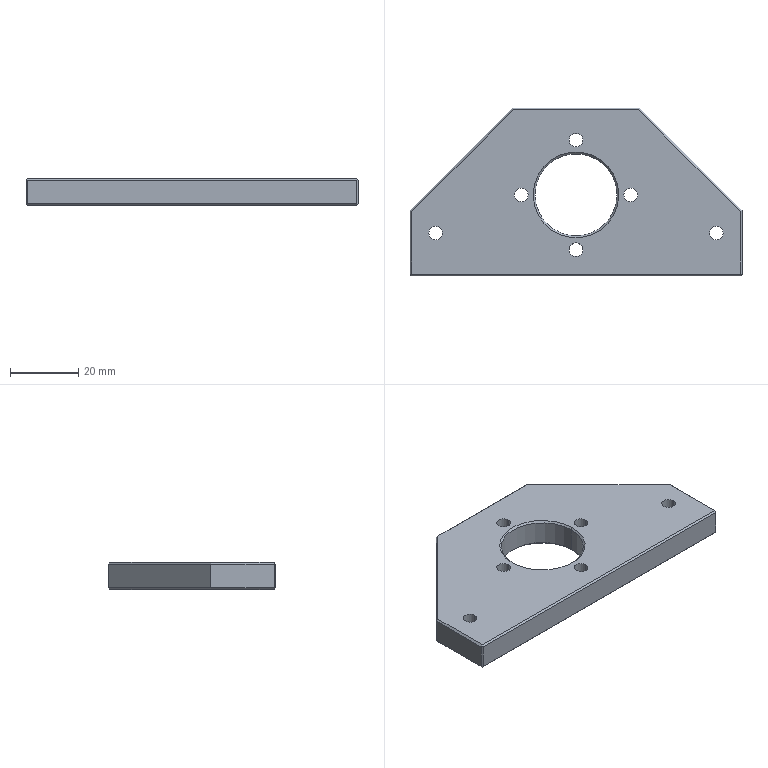Part | Creo | features DATUM PLANE 3, CURVE 2, CHAMFER 1, COORDINATE SYSTEM 1, CUT 1, PROTRUSION 1 | 1 solid | 46 faces | box 97 x 49 x 8 mm | volume 26205 mm3 | plane 24 | cylinder 18 | cone 4 | commonest cylinder face diameters 4 x12 7.464 x4 24 x2
STEP:
#1=CARTESIAN_POINT('',(0.,0.,0.));
#2=DIRECTION('',(0.,0.,1.));
#3=DIRECTION('',(1.,0.,0.));
#4=AXIS2_PLACEMENT_3D('',#1,#2,#3);
#5=CARTESIAN_POINT('',(48.,0.5,0.));
#6=VERTEX_POINT('',#5);
#7=CARTESIAN_POINT('',(-48.,0.5,0.));
#8=VERTEX_POINT('',#7);
#9=CARTESIAN_POINT('',(48.,0.5,0.));
#10=DIRECTION('',(-1.,0.,0.));
#11=VECTOR('',#10,96.);
#12=LINE('',#9,#11);
#13=EDGE_CURVE('',#6,#8,#12,.T.);
#14=ORIENTED_EDGE('',*,*,#13,.F.);
#15=CARTESIAN_POINT('',(48.,18.793,0.));
#16=VERTEX_POINT('',#15);
#17=CARTESIAN_POINT('',(48.,18.793,0.));
#18=DIRECTION('',(0.,-1.,0.));
#19=VECTOR('',#18,18.293);
#20=LINE('',#17,#19);
#21=EDGE_CURVE('',#16,#6,#20,.T.);
#22=ORIENTED_EDGE('',*,*,#21,.F.);
#23=CARTESIAN_POINT('',(18.293,48.5,0.));
#24=VERTEX_POINT('',#23);
#25=CARTESIAN_POINT('',(18.293,48.5,0.));
#26=DIRECTION('',(0.7071,-0.7071,0.));
#27=VECTOR('',#26,42.012);
#28=LINE('',#25,#27);
#29=EDGE_CURVE('',#24,#16,#28,.T.);
#30=ORIENTED_EDGE('',*,*,#29,.F.);
#31=CARTESIAN_POINT('',(-18.293,48.5,0.));
#32=VERTEX_POINT('',#31);
#33=CARTESIAN_POINT('',(-18.293,48.5,0.));
#34=DIRECTION('',(1.,0.,0.));
#35=VECTOR('',#34,36.586);
#36=LINE('',#33,#35);
#37=EDGE_CURVE('',#32,#24,#36,.T.);
#38=ORIENTED_EDGE('',*,*,#37,.F.);
#39=CARTESIAN_POINT('',(-48.,18.793,0.));
#40=VERTEX_POINT('',#39);
#41=CARTESIAN_POINT('',(-48.,18.793,0.));
#42=DIRECTION('',(0.7071,0.7071,0.));
#43=VECTOR('',#42,42.012);
#44=LINE('',#41,#43);
#45=EDGE_CURVE('',#40,#32,#44,.T.);
#46=ORIENTED_EDGE('',*,*,#45,.F.);
#47=CARTESIAN_POINT('',(-48.,0.5,0.));
#48=DIRECTION('',(0.,1.,0.));
#49=VECTOR('',#48,18.293);
#50=LINE('',#47,#49);
#51=EDGE_CURVE('',#8,#40,#50,.T.);
#52=ORIENTED_EDGE('',*,*,#51,.F.);
#53=EDGE_LOOP('',(#14,#22,#30,#38,#46,#52));
#54=FACE_OUTER_BOUND('',#53,.F.);
#55=CARTESIAN_POINT('',(2.,39.66,0.));
#56=VERTEX_POINT('',#55);
#57=CARTESIAN_POINT('',(-2.,39.66,0.));
#58=VERTEX_POINT('',#57);
#59=CARTESIAN_POINT('',(0.,39.66,0.));
#60=DIRECTION('',(0.,0.,-1.));
#61=DIRECTION('',(1.,0.,0.));
#62=AXIS2_PLACEMENT_3D('',#59,#60,#61);
#63=CIRCLE('',#62,2.);
#64=EDGE_CURVE('',#56,#58,#63,.T.);
#65=ORIENTED_EDGE('',*,*,#64,.T.);
#66=CARTESIAN_POINT('',(0.,39.66,0.));
#67=DIRECTION('',(0.,0.,-1.));
#68=DIRECTION('',(-1.,0.,0.));
#69=AXIS2_PLACEMENT_3D('',#66,#67,#68);
#70=CIRCLE('',#69,2.);
#71=EDGE_CURVE('',#58,#56,#70,.T.);
#72=ORIENTED_EDGE('',*,*,#71,.T.);
#73=EDGE_LOOP('',(#65,#72));
#74=FACE_BOUND('',#73,.F.);
#75=CARTESIAN_POINT('',(-14.,23.66,0.));
#76=VERTEX_POINT('',#75);
#77=CARTESIAN_POINT('',(-18.,23.66,0.));
#78=VERTEX_POINT('',#77);
#79=CARTESIAN_POINT('',(-16.,23.66,0.));
#80=DIRECTION('',(0.,0.,-1.));
#81=DIRECTION('',(1.,0.,0.));
#82=AXIS2_PLACEMENT_3D('',#79,#80,#81);
#83=CIRCLE('',#82,2.);
#84=EDGE_CURVE('',#76,#78,#83,.T.);
#85=ORIENTED_EDGE('',*,*,#84,.T.);
#86=CARTESIAN_POINT('',(-16.,23.66,0.));
#87=DIRECTION('',(0.,0.,-1.));
#88=DIRECTION('',(-1.,0.,0.));
#89=AXIS2_PLACEMENT_3D('',#86,#87,#88);
#90=CIRCLE('',#89,2.);
#91=EDGE_CURVE('',#78,#76,#90,.T.);
#92=ORIENTED_EDGE('',*,*,#91,.T.);
#93=EDGE_LOOP('',(#85,#92));
#94=FACE_BOUND('',#93,.F.);
#95=CARTESIAN_POINT('',(2.,7.66,0.));
#96=VERTEX_POINT('',#95);
#97=CARTESIAN_POINT('',(-2.,7.66,0.));
#98=VERTEX_POINT('',#97);
#99=CARTESIAN_POINT('',(0.,7.66,0.));
#100=DIRECTION('',(0.,0.,-1.));
#101=DIRECTION('',(1.,0.,0.));
#102=AXIS2_PLACEMENT_3D('',#99,#100,#101);
#103=CIRCLE('',#102,2.);
#104=EDGE_CURVE('',#96,#98,#103,.T.);
#105=ORIENTED_EDGE('',*,*,#104,.T.);
#106=CARTESIAN_POINT('',(0.,7.66,0.));
#107=DIRECTION('',(0.,0.,-1.));
#108=DIRECTION('',(-1.,0.,0.));
#109=AXIS2_PLACEMENT_3D('',#106,#107,#108);
#110=CIRCLE('',#109,2.);
#111=EDGE_CURVE('',#98,#96,#110,.T.);
#112=ORIENTED_EDGE('',*,*,#111,.T.);
#113=EDGE_LOOP('',(#105,#112));
#114=FACE_BOUND('',#113,.F.);
#115=CARTESIAN_POINT('',(-44.732,12.5,0.));
#116=VERTEX_POINT('',#115);
#117=CARTESIAN_POINT('',(-37.268,12.5,0.));
#118=VERTEX_POINT('',#117);
#119=CARTESIAN_POINT('',(-41.,12.5,0.));
#120=DIRECTION('',(0.,0.,-1.));
#121=DIRECTION('',(-1.,0.,0.));
#122=AXIS2_PLACEMENT_3D('',#119,#120,#121);
#123=CIRCLE('',#122,3.732);
#124=EDGE_CURVE('',#116,#118,#123,.T.);
#125=ORIENTED_EDGE('',*,*,#124,.T.);
#126=CARTESIAN_POINT('',(-41.,12.5,0.));
#127=DIRECTION('',(0.,0.,-1.));
#128=DIRECTION('',(1.,0.,0.));
#129=AXIS2_PLACEMENT_3D('',#126,#127,#128);
#130=CIRCLE('',#129,3.732);
#131=EDGE_CURVE('',#118,#116,#130,.T.);
#132=ORIENTED_EDGE('',*,*,#131,.T.);
#133=EDGE_LOOP('',(#125,#132));
#134=FACE_BOUND('',#133,.F.);
#135=CARTESIAN_POINT('',(37.268,12.5,0.));
#136=VERTEX_POINT('',#135);
#137=CARTESIAN_POINT('',(44.732,12.5,0.));
#138=VERTEX_POINT('',#137);
#139=CARTESIAN_POINT('',(41.,12.5,0.));
#140=DIRECTION('',(0.,0.,-1.));
#141=DIRECTION('',(-1.,0.,0.));
#142=AXIS2_PLACEMENT_3D('',#139,#140,#141);
#143=CIRCLE('',#142,3.732);
#144=EDGE_CURVE('',#136,#138,#143,.T.);
#145=ORIENTED_EDGE('',*,*,#144,.T.);
#146=CARTESIAN_POINT('',(41.,12.5,0.));
#147=DIRECTION('',(0.,0.,-1.));
#148=DIRECTION('',(1.,0.,0.));
#149=AXIS2_PLACEMENT_3D('',#146,#147,#148);
#150=CIRCLE('',#149,3.732);
#151=EDGE_CURVE('',#138,#136,#150,.T.);
#152=ORIENTED_EDGE('',*,*,#151,.T.);
#153=EDGE_LOOP('',(#145,#152));
#154=FACE_BOUND('',#153,.F.);
#155=CARTESIAN_POINT('',(18.,23.66,0.));
#156=VERTEX_POINT('',#155);
#157=CARTESIAN_POINT('',(14.,23.66,0.));
#158=VERTEX_POINT('',#157);
#159=CARTESIAN_POINT('',(16.,23.66,0.));
#160=DIRECTION('',(0.,0.,-1.));
#161=DIRECTION('',(1.,0.,0.));
#162=AXIS2_PLACEMENT_3D('',#159,#160,#161);
#163=CIRCLE('',#162,2.);
#164=EDGE_CURVE('',#156,#158,#163,.T.);
#165=ORIENTED_EDGE('',*,*,#164,.T.);
#166=CARTESIAN_POINT('',(16.,23.66,0.));
#167=DIRECTION('',(0.,0.,-1.));
#168=DIRECTION('',(-1.,0.,0.));
#169=AXIS2_PLACEMENT_3D('',#166,#167,#168);
#170=CIRCLE('',#169,2.);
#171=EDGE_CURVE('',#158,#156,#170,.T.);
#172=ORIENTED_EDGE('',*,*,#171,.T.);
#173=EDGE_LOOP('',(#165,#172));
#174=FACE_BOUND('',#173,.F.);
#175=CARTESIAN_POINT('',(12.5,23.66,0.));
#176=VERTEX_POINT('',#175);
#177=CARTESIAN_POINT('',(-12.5,23.66,0.));
#178=VERTEX_POINT('',#177);
#179=CARTESIAN_POINT('',(0.,23.66,0.));
#180=DIRECTION('',(0.,0.,1.));
#181=DIRECTION('',(1.,0.,0.));
#182=AXIS2_PLACEMENT_3D('',#179,#180,#181);
#183=CIRCLE('',#182,12.5);
#184=EDGE_CURVE('',#176,#178,#183,.T.);
#185=ORIENTED_EDGE('',*,*,#184,.F.);
#186=CARTESIAN_POINT('',(0.,23.66,0.));
#187=DIRECTION('',(0.,0.,1.));
#188=DIRECTION('',(-1.,0.,0.));
#189=AXIS2_PLACEMENT_3D('',#186,#187,#188);
#190=CIRCLE('',#189,12.5);
#191=EDGE_CURVE('',#178,#176,#190,.T.);
#192=ORIENTED_EDGE('',*,*,#191,.F.);
#193=EDGE_LOOP('',(#185,#192));
#194=FACE_BOUND('',#193,.F.);
#195=CARTESIAN_POINT('',(0.,0.,0.));
#196=DIRECTION('',(0.,0.,1.));
#197=DIRECTION('',(1.,0.,0.));
#198=AXIS2_PLACEMENT_3D('',#195,#196,#197);
#199=PLANE('',#198);
#200=ADVANCED_FACE('',(#54,#74,#94,#114,#134,#154,#174,#194),#199,.F.);
#201=ORIENTED_EDGE('',*,*,#164,.F.);
#202=CARTESIAN_POINT('',(18.,23.66,8.));
#203=VERTEX_POINT('',#202);
#204=CARTESIAN_POINT('',(18.,23.66,0.));
#205=DIRECTION('',(0.,0.,1.));
#206=VECTOR('',#205,8.);
#207=LINE('',#204,#206);
#208=EDGE_CURVE('',#156,#203,#207,.T.);
#209=ORIENTED_EDGE('',*,*,#208,.T.);
#210=CARTESIAN_POINT('',(14.,23.66,8.));
#211=VERTEX_POINT('',#210);
#212=CARTESIAN_POINT('',(16.,23.66,8.));
#213=DIRECTION('',(0.,0.,-1.));
#214=DIRECTION('',(1.,0.,0.));
#215=AXIS2_PLACEMENT_3D('',#212,#213,#214);
#216=CIRCLE('',#215,2.);
#217=EDGE_CURVE('',#203,#211,#216,.T.);
#218=ORIENTED_EDGE('',*,*,#217,.T.);
#219=CARTESIAN_POINT('',(14.,23.66,0.));
#220=DIRECTION('',(0.,0.,1.));
#221=VECTOR('',#220,8.);
#222=LINE('',#219,#221);
#223=EDGE_CURVE('',#158,#211,#222,.T.);
#224=ORIENTED_EDGE('',*,*,#223,.F.);
#225=EDGE_LOOP('',(#201,#209,#218,#224));
#226=FACE_OUTER_BOUND('',#225,.F.);
#227=CARTESIAN_POINT('',(16.,23.66,0.));
#228=DIRECTION('',(0.,0.,1.));
#229=DIRECTION('',(1.,0.,0.));
#230=AXIS2_PLACEMENT_3D('',#227,#228,#229);
#231=CYLINDRICAL_SURFACE('',#230,2.);
#232=ADVANCED_FACE('',(#226),#231,.F.);
#233=ORIENTED_EDGE('',*,*,#171,.F.);
#234=ORIENTED_EDGE('',*,*,#223,.T.);
#235=CARTESIAN_POINT('',(16.,23.66,8.));
#236=DIRECTION('',(0.,0.,-1.));
#237=DIRECTION('',(-1.,0.,0.));
#238=AXIS2_PLACEMENT_3D('',#235,#236,#237);
#239=CIRCLE('',#238,2.);
#240=EDGE_CURVE('',#211,#203,#239,.T.);
#241=ORIENTED_EDGE('',*,*,#240,.T.);
#242=ORIENTED_EDGE('',*,*,#208,.F.);
#243=EDGE_LOOP('',(#233,#234,#241,#242));
#244=FACE_OUTER_BOUND('',#243,.F.);
#245=CARTESIAN_POINT('',(16.,23.66,0.));
#246=DIRECTION('',(0.,0.,1.));
#247=DIRECTION('',(1.,0.,0.));
#248=AXIS2_PLACEMENT_3D('',#245,#246,#247);
#249=CYLINDRICAL_SURFACE('',#248,2.);
#250=ADVANCED_FACE('',(#244),#249,.F.);
#251=CARTESIAN_POINT('',(-48.,0.5,8.));
#252=VERTEX_POINT('',#251);
#253=CARTESIAN_POINT('',(48.,0.5,8.));
#254=VERTEX_POINT('',#253);
#255=CARTESIAN_POINT('',(-48.,0.5,8.));
#256=DIRECTION('',(1.,0.,0.));
#257=VECTOR('',#256,96.);
#258=LINE('',#255,#257);
#259=EDGE_CURVE('',#252,#254,#258,.T.);
#260=ORIENTED_EDGE('',*,*,#259,.F.);
#261=CARTESIAN_POINT('',(-48.,18.793,8.));
#262=VERTEX_POINT('',#261);
#263=CARTESIAN_POINT('',(-48.,18.793,8.));
#264=DIRECTION('',(0.,-1.,0.));
#265=VECTOR('',#264,18.293);
#266=LINE('',#263,#265);
#267=EDGE_CURVE('',#262,#252,#266,.T.);
#268=ORIENTED_EDGE('',*,*,#267,.F.);
#269=CARTESIAN_POINT('',(-18.293,48.5,8.));
#270=VERTEX_POINT('',#269);
#271=CARTESIAN_POINT('',(-18.293,48.5,8.));
#272=DIRECTION('',(-0.7071,-0.7071,0.));
#273=VECTOR('',#272,42.012);
#274=LINE('',#271,#273);
#275=EDGE_CURVE('',#270,#262,#274,.T.);
#276=ORIENTED_EDGE('',*,*,#275,.F.);
#277=CARTESIAN_POINT('',(18.293,48.5,8.));
#278=VERTEX_POINT('',#277);
#279=CARTESIAN_POINT('',(18.293,48.5,8.));
#280=DIRECTION('',(-1.,0.,0.));
#281=VECTOR('',#280,36.586);
#282=LINE('',#279,#281);
#283=EDGE_CURVE('',#278,#270,#282,.T.);
#284=ORIENTED_EDGE('',*,*,#283,.F.);
#285=CARTESIAN_POINT('',(48.,18.793,8.));
#286=VERTEX_POINT('',#285);
#287=CARTESIAN_POINT('',(48.,18.793,8.));
#288=DIRECTION('',(-0.7071,0.7071,0.));
#289=VECTOR('',#288,42.012);
#290=LINE('',#287,#289);
#291=EDGE_CURVE('',#286,#278,#290,.T.);
#292=ORIENTED_EDGE('',*,*,#291,.F.);
#293=CARTESIAN_POINT('',(48.,0.5,8.));
#294=DIRECTION('',(0.,1.,0.));
#295=VECTOR('',#294,18.293);
#296=LINE('',#293,#295);
#297=EDGE_CURVE('',#254,#286,#296,.T.);
#298=ORIENTED_EDGE('',*,*,#297,.F.);
#299=EDGE_LOOP('',(#260,#268,#276,#284,#292,#298));
#300=FACE_OUTER_BOUND('',#299,.F.);
#301=CARTESIAN_POINT('',(43.,12.5,8.));
#302=VERTEX_POINT('',#301);
#303=CARTESIAN_POINT('',(39.,12.5,8.));
#304=VERTEX_POINT('',#303);
#305=CARTESIAN_POINT('',(41.,12.5,8.));
#306=DIRECTION('',(0.,0.,-1.));
#307=DIRECTION('',(1.,0.,0.));
#308=AXIS2_PLACEMENT_3D('',#305,#306,#307);
#309=CIRCLE('',#308,2.);
#310=EDGE_CURVE('',#302,#304,#309,.T.);
#311=ORIENTED_EDGE('',*,*,#310,.F.);
#312=CARTESIAN_POINT('',(41.,12.5,8.));
#313=DIRECTION('',(0.,0.,-1.));
#314=DIRECTION('',(-1.,0.,0.));
#315=AXIS2_PLACEMENT_3D('',#312,#313,#314);
#316=CIRCLE('',#315,2.);
#317=EDGE_CURVE('',#304,#302,#316,.T.);
#318=ORIENTED_EDGE('',*,*,#317,.F.);
#319=EDGE_LOOP('',(#311,#318));
#320=FACE_BOUND('',#319,.F.);
#321=ORIENTED_EDGE('',*,*,#217,.F.);
#322=ORIENTED_EDGE('',*,*,#240,.F.);
#323=EDGE_LOOP('',(#321,#322));
#324=FACE_BOUND('',#323,.F.);
#325=CARTESIAN_POINT('',(2.,39.66,8.));
#326=VERTEX_POINT('',#325);
#327=CARTESIAN_POINT('',(-2.,39.66,8.));
#328=VERTEX_POINT('',#327);
#329=CARTESIAN_POINT('',(0.,39.66,8.));
#330=DIRECTION('',(0.,0.,-1.));
#331=DIRECTION('',(1.,0.,0.));
#332=AXIS2_PLACEMENT_3D('',#329,#330,#331);
#333=CIRCLE('',#332,2.);
#334=EDGE_CURVE('',#326,#328,#333,.T.);
#335=ORIENTED_EDGE('',*,*,#334,.F.);
#336=CARTESIAN_POINT('',(0.,39.66,8.));
#337=DIRECTION('',(0.,0.,-1.));
#338=DIRECTION('',(-1.,0.,0.));
#339=AXIS2_PLACEMENT_3D('',#336,#337,#338);
#340=CIRCLE('',#339,2.);
#341=EDGE_CURVE('',#328,#326,#340,.T.);
#342=ORIENTED_EDGE('',*,*,#341,.F.);
#343=EDGE_LOOP('',(#335,#342));
#344=FACE_BOUND('',#343,.F.);
#345=CARTESIAN_POINT('',(-14.,23.66,8.));
#346=VERTEX_POINT('',#345);
#347=CARTESIAN_POINT('',(-18.,23.66,8.));
#348=VERTEX_POINT('',#347);
#349=CARTESIAN_POINT('',(-16.,23.66,8.));
#350=DIRECTION('',(0.,0.,-1.));
#351=DIRECTION('',(1.,0.,0.));
#352=AXIS2_PLACEMENT_3D('',#349,#350,#351);
#353=CIRCLE('',#352,2.);
#354=EDGE_CURVE('',#346,#348,#353,.T.);
#355=ORIENTED_EDGE('',*,*,#354,.F.);
#356=CARTESIAN_POINT('',(-16.,23.66,8.));
#357=DIRECTION('',(0.,0.,-1.));
#358=DIRECTION('',(-1.,0.,0.));
#359=AXIS2_PLACEMENT_3D('',#356,#357,#358);
#360=CIRCLE('',#359,2.);
#361=EDGE_CURVE('',#348,#346,#360,.T.);
#362=ORIENTED_EDGE('',*,*,#361,.F.);
#363=EDGE_LOOP('',(#355,#362));
#364=FACE_BOUND('',#363,.F.);
#365=CARTESIAN_POINT('',(2.,7.66,8.));
#366=VERTEX_POINT('',#365);
#367=CARTESIAN_POINT('',(-2.,7.66,8.));
#368=VERTEX_POINT('',#367);
#369=CARTESIAN_POINT('',(0.,7.66,8.));
#370=DIRECTION('',(0.,0.,-1.));
#371=DIRECTION('',(1.,0.,0.));
#372=AXIS2_PLACEMENT_3D('',#369,#370,#371);
#373=CIRCLE('',#372,2.);
#374=EDGE_CURVE('',#366,#368,#373,.T.);
#375=ORIENTED_EDGE('',*,*,#374,.F.);
#376=CARTESIAN_POINT('',(0.,7.66,8.));
#377=DIRECTION('',(0.,0.,-1.));
#378=DIRECTION('',(-1.,0.,0.));
#379=AXIS2_PLACEMENT_3D('',#376,#377,#378);
#380=CIRCLE('',#379,2.);
#381=EDGE_CURVE('',#368,#366,#380,.T.);
#382=ORIENTED_EDGE('',*,*,#381,.F.);
#383=EDGE_LOOP('',(#375,#382));
#384=FACE_BOUND('',#383,.F.);
#385=CARTESIAN_POINT('',(-39.,12.5,8.));
#386=VERTEX_POINT('',#385);
#387=CARTESIAN_POINT('',(-43.,12.5,8.));
#388=VERTEX_POINT('',#387);
#389=CARTESIAN_POINT('',(-41.,12.5,8.));
#390=DIRECTION('',(0.,0.,-1.));
#391=DIRECTION('',(1.,0.,0.));
#392=AXIS2_PLACEMENT_3D('',#389,#390,#391);
#393=CIRCLE('',#392,2.);
#394=EDGE_CURVE('',#386,#388,#393,.T.);
#395=ORIENTED_EDGE('',*,*,#394,.F.);
#396=CARTESIAN_POINT('',(-41.,12.5,8.));
#397=DIRECTION('',(0.,0.,-1.));
#398=DIRECTION('',(-1.,0.,0.));
#399=AXIS2_PLACEMENT_3D('',#396,#397,#398);
#400=CIRCLE('',#399,2.);
#401=EDGE_CURVE('',#388,#386,#400,.T.);
#402=ORIENTED_EDGE('',*,*,#401,.F.);
#403=EDGE_LOOP('',(#395,#402));
#404=FACE_BOUND('',#403,.F.);
#405=CARTESIAN_POINT('',(-12.5,23.66,8.));
#406=VERTEX_POINT('',#405);
#407=CARTESIAN_POINT('',(12.5,23.66,8.));
#408=VERTEX_POINT('',#407);
#409=CARTESIAN_POINT('',(0.,23.66,8.));
#410=DIRECTION('',(0.,0.,-1.));
#411=DIRECTION('',(-1.,0.,0.));
#412=AXIS2_PLACEMENT_3D('',#409,#410,#411);
#413=CIRCLE('',#412,12.5);
#414=EDGE_CURVE('',#406,#408,#413,.T.);
#415=ORIENTED_EDGE('',*,*,#414,.F.);
#416=CARTESIAN_POINT('',(0.,23.66,8.));
#417=DIRECTION('',(0.,0.,-1.));
#418=DIRECTION('',(1.,0.,0.));
#419=AXIS2_PLACEMENT_3D('',#416,#417,#418);
#420=CIRCLE('',#419,12.5);
#421=EDGE_CURVE('',#408,#406,#420,.T.);
#422=ORIENTED_EDGE('',*,*,#421,.F.);
#423=EDGE_LOOP('',(#415,#422));
#424=FACE_BOUND('',#423,.F.);
#425=CARTESIAN_POINT('',(0.,0.,8.));
#426=DIRECTION('',(0.,0.,1.));
#427=DIRECTION('',(1.,0.,0.));
#428=AXIS2_PLACEMENT_3D('',#425,#426,#427);
#429=PLANE('',#428);
#430=ADVANCED_FACE('',(#300,#320,#324,#344,#364,#384,#404,#424),#429,.T.);
#431=CARTESIAN_POINT('',(-43.,12.5,5.));
#432=VERTEX_POINT('',#431);
#433=CARTESIAN_POINT('',(-39.,12.5,5.));
#434=VERTEX_POINT('',#433);
#435=CARTESIAN_POINT('',(-41.,12.5,5.));
#436=DIRECTION('',(0.,0.,1.));
#437=DIRECTION('',(-1.,0.,0.));
#438=AXIS2_PLACEMENT_3D('',#435,#436,#437);
#439=CIRCLE('',#438,2.);
#440=EDGE_CURVE('',#432,#434,#439,.T.);
#441=ORIENTED_EDGE('',*,*,#440,.T.);
#442=CARTESIAN_POINT('',(-39.,12.5,5.));
#443=DIRECTION('',(0.,0.,1.));
#444=VECTOR('',#443,3.);
#445=LINE('',#442,#444);
#446=EDGE_CURVE('',#434,#386,#445,.T.);
#447=ORIENTED_EDGE('',*,*,#446,.T.);
#448=ORIENTED_EDGE('',*,*,#394,.T.);
#449=CARTESIAN_POINT('',(-43.,12.5,5.));
#450=DIRECTION('',(0.,0.,1.));
#451=VECTOR('',#450,3.);
#452=LINE('',#449,#451);
#453=EDGE_CURVE('',#432,#388,#452,.T.);
#454=ORIENTED_EDGE('',*,*,#453,.F.);
#455=EDGE_LOOP('',(#441,#447,#448,#454));
#456=FACE_OUTER_BOUND('',#455,.F.);
#457=CARTESIAN_POINT('',(-41.,12.5,0.));
#458=DIRECTION('',(0.,0.,1.));
#459=DIRECTION('',(1.,0.,0.));
#460=AXIS2_PLACEMENT_3D('',#457,#458,#459);
#461=CYLINDRICAL_SURFACE('',#460,2.);
#462=ADVANCED_FACE('',(#456),#461,.F.);
#463=CARTESIAN_POINT('',(-44.732,12.5,5.));
#464=VERTEX_POINT('',#463);
#465=CARTESIAN_POINT('',(-37.268,12.5,5.));
#466=VERTEX_POINT('',#465);
#467=CARTESIAN_POINT('',(-41.,12.5,5.));
#468=DIRECTION('',(0.,0.,-1.));
#469=DIRECTION('',(-1.,0.,0.));
#470=AXIS2_PLACEMENT_3D('',#467,#468,#469);
#471=CIRCLE('',#470,3.732);
#472=EDGE_CURVE('',#464,#466,#471,.T.);
#473=ORIENTED_EDGE('',*,*,#472,.F.);
#474=CARTESIAN_POINT('',(-41.,12.5,5.));
#475=DIRECTION('',(0.,0.,-1.));
#476=DIRECTION('',(1.,0.,0.));
#477=AXIS2_PLACEMENT_3D('',#474,#475,#476);
#478=CIRCLE('',#477,3.732);
#479=EDGE_CURVE('',#466,#464,#478,.T.);
#480=ORIENTED_EDGE('',*,*,#479,.F.);
#481=EDGE_LOOP('',(#473,#480));
#482=FACE_OUTER_BOUND('',#481,.F.);
#483=ORIENTED_EDGE('',*,*,#440,.F.);
#484=CARTESIAN_POINT('',(-41.,12.5,5.));
#485=DIRECTION('',(0.,0.,1.));
#486=DIRECTION('',(1.,0.,0.));
#487=AXIS2_PLACEMENT_3D('',#484,#485,#486);
#488=CIRCLE('',#487,2.);
#489=EDGE_CURVE('',#434,#432,#488,.T.);
#490=ORIENTED_EDGE('',*,*,#489,.F.);
#491=EDGE_LOOP('',(#483,#490));
#492=FACE_BOUND('',#491,.F.);
#493=CARTESIAN_POINT('',(0.,0.,5.));
#494=DIRECTION('',(0.,0.,-1.));
#495=DIRECTION('',(-1.,0.,0.));
#496=AXIS2_PLACEMENT_3D('',#493,#494,#495);
#497=PLANE('',#496);
#498=ADVANCED_FACE('',(#482,#492),#497,.T.);
#499=CARTESIAN_POINT('',(37.268,12.5,5.));
#500=VERTEX_POINT('',#499);
#501=CARTESIAN_POINT('',(44.732,12.5,5.));
#502=VERTEX_POINT('',#501);
#503=CARTESIAN_POINT('',(41.,12.5,5.));
#504=DIRECTION('',(0.,0.,-1.));
#505=DIRECTION('',(-1.,0.,0.));
#506=AXIS2_PLACEMENT_3D('',#503,#504,#505);
#507=CIRCLE('',#506,3.732);
#508=EDGE_CURVE('',#500,#502,#507,.T.);
#509=ORIENTED_EDGE('',*,*,#508,.F.);
#510=CARTESIAN_POINT('',(41.,12.5,5.));
#511=DIRECTION('',(0.,0.,-1.));
#512=DIRECTION('',(1.,0.,0.));
#513=AXIS2_PLACEMENT_3D('',#510,#511,#512);
#514=CIRCLE('',#513,3.732);
#515=EDGE_CURVE('',#502,#500,#514,.T.);
#516=ORIENTED_EDGE('',*,*,#515,.F.);
#517=EDGE_LOOP('',(#509,#516));
#518=FACE_OUTER_BOUND('',#517,.F.);
#519=CARTESIAN_POINT('',(39.,12.5,5.));
#520=VERTEX_POINT('',#519);
#521=CARTESIAN_POINT('',(43.,12.5,5.));
#522=VERTEX_POINT('',#521);
#523=CARTESIAN_POINT('',(41.,12.5,5.));
#524=DIRECTION('',(0.,0.,1.));
#525=DIRECTION('',(-1.,0.,0.));
#526=AXIS2_PLACEMENT_3D('',#523,#524,#525);
#527=CIRCLE('',#526,2.);
#528=EDGE_CURVE('',#520,#522,#527,.T.);
#529=ORIENTED_EDGE('',*,*,#528,.F.);
#530=CARTESIAN_POINT('',(41.,12.5,5.));
#531=DIRECTION('',(0.,0.,1.));
#532=DIRECTION('',(1.,0.,0.));
#533=AXIS2_PLACEMENT_3D('',#530,#531,#532);
#534=CIRCLE('',#533,2.);
#535=EDGE_CURVE('',#522,#520,#534,.T.);
#536=ORIENTED_EDGE('',*,*,#535,.F.);
#537=EDGE_LOOP('',(#529,#536));
#538=FACE_BOUND('',#537,.F.);
#539=CARTESIAN_POINT('',(0.,0.,5.));
#540=DIRECTION('',(0.,0.,-1.));
#541=DIRECTION('',(-1.,0.,0.));
#542=AXIS2_PLACEMENT_3D('',#539,#540,#541);
#543=PLANE('',#542);
#544=ADVANCED_FACE('',(#518,#538),#543,.T.);
#545=ORIENTED_EDGE('',*,*,#124,.F.);
#546=CARTESIAN_POINT('',(-44.732,12.5,0.));
#547=DIRECTION('',(0.,0.,1.));
#548=VECTOR('',#547,5.);
#549=LINE('',#546,#548);
#550=EDGE_CURVE('',#116,#464,#549,.T.);
#551=ORIENTED_EDGE('',*,*,#550,.T.);
#552=ORIENTED_EDGE('',*,*,#472,.T.);
#553=CARTESIAN_POINT('',(-37.268,12.5,0.));
#554=DIRECTION('',(0.,0.,1.));
#555=VECTOR('',#554,5.);
#556=LINE('',#553,#555);
#557=EDGE_CURVE('',#118,#466,#556,.T.);
#558=ORIENTED_EDGE('',*,*,#557,.F.);
#559=EDGE_LOOP('',(#545,#551,#552,#558));
#560=FACE_OUTER_BOUND('',#559,.F.);
#561=CARTESIAN_POINT('',(-41.,12.5,0.));
#562=DIRECTION('',(0.,0.,-1.));
#563=DIRECTION('',(-1.,0.,0.));
#564=AXIS2_PLACEMENT_3D('',#561,#562,#563);
#565=CYLINDRICAL_SURFACE('',#564,3.732);
#566=ADVANCED_FACE('',(#560),#565,.F.);
#567=ORIENTED_EDGE('',*,*,#131,.F.);
#568=ORIENTED_EDGE('',*,*,#557,.T.);
#569=ORIENTED_EDGE('',*,*,#479,.T.);
#570=ORIENTED_EDGE('',*,*,#550,.F.);
#571=EDGE_LOOP('',(#567,#568,#569,#570));
#572=FACE_OUTER_BOUND('',#571,.F.);
#573=CARTESIAN_POINT('',(-41.,12.5,0.));
#574=DIRECTION('',(0.,0.,-1.));
#575=DIRECTION('',(-1.,0.,0.));
#576=AXIS2_PLACEMENT_3D('',#573,#574,#575);
#577=CYLINDRICAL_SURFACE('',#576,3.732);
#578=ADVANCED_FACE('',(#572),#577,.F.);
#579=ORIENTED_EDGE('',*,*,#144,.F.);
#580=CARTESIAN_POINT('',(37.268,12.5,0.));
#581=DIRECTION('',(0.,0.,1.));
#582=VECTOR('',#581,5.);
#583=LINE('',#580,#582);
#584=EDGE_CURVE('',#136,#500,#583,.T.);
#585=ORIENTED_EDGE('',*,*,#584,.T.);
#586=ORIENTED_EDGE('',*,*,#508,.T.);
#587=CARTESIAN_POINT('',(44.732,12.5,0.));
#588=DIRECTION('',(0.,0.,1.));
#589=VECTOR('',#588,5.);
#590=LINE('',#587,#589);
#591=EDGE_CURVE('',#138,#502,#590,.T.);
#592=ORIENTED_EDGE('',*,*,#591,.F.);
#593=EDGE_LOOP('',(#579,#585,#586,#592));
#594=FACE_OUTER_BOUND('',#593,.F.);
#595=CARTESIAN_POINT('',(41.,12.5,0.));
#596=DIRECTION('',(0.,0.,-1.));
#597=DIRECTION('',(-1.,0.,0.));
#598=AXIS2_PLACEMENT_3D('',#595,#596,#597);
#599=CYLINDRICAL_SURFACE('',#598,3.732);
#600=ADVANCED_FACE('',(#594),#599,.F.);
#601=ORIENTED_EDGE('',*,*,#151,.F.);
#602=ORIENTED_EDGE('',*,*,#591,.T.);
#603=ORIENTED_EDGE('',*,*,#515,.T.);
#604=ORIENTED_EDGE('',*,*,#584,.F.);
#605=EDGE_LOOP('',(#601,#602,#603,#604));
#606=FACE_OUTER_BOUND('',#605,.F.);
#607=CARTESIAN_POINT('',(41.,12.5,0.));
#608=DIRECTION('',(0.,0.,-1.));
#609=DIRECTION('',(-1.,0.,0.));
#610=AXIS2_PLACEMENT_3D('',#607,#608,#609);
#611=CYLINDRICAL_SURFACE('',#610,3.732);
#612=ADVANCED_FACE('',(#606),#611,.F.);
#613=ORIENTED_EDGE('',*,*,#489,.T.);
#614=ORIENTED_EDGE('',*,*,#453,.T.);
#615=ORIENTED_EDGE('',*,*,#401,.T.);
#616=ORIENTED_EDGE('',*,*,#446,.F.);
#617=EDGE_LOOP('',(#613,#614,#615,#616));
#618=FACE_OUTER_BOUND('',#617,.F.);
#619=CARTESIAN_POINT('',(-41.,12.5,0.));
#620=DIRECTION('',(0.,0.,1.));
#621=DIRECTION('',(1.,0.,0.));
#622=AXIS2_PLACEMENT_3D('',#619,#620,#621);
#623=CYLINDRICAL_SURFACE('',#622,2.);
#624=ADVANCED_FACE('',(#618),#623,.F.);
#625=ORIENTED_EDGE('',*,*,#528,.T.);
#626=CARTESIAN_POINT('',(43.,12.5,5.));
#627=DIRECTION('',(0.,0.,1.));
#628=VECTOR('',#627,3.);
#629=LINE('',#626,#628);
#630=EDGE_CURVE('',#522,#302,#629,.T.);
#631=ORIENTED_EDGE('',*,*,#630,.T.);
#632=ORIENTED_EDGE('',*,*,#310,.T.);
#633=CARTESIAN_POINT('',(39.,12.5,5.));
#634=DIRECTION('',(0.,0.,1.));
#635=VECTOR('',#634,3.);
#636=LINE('',#633,#635);
#637=EDGE_CURVE('',#520,#304,#636,.T.);
#638=ORIENTED_EDGE('',*,*,#637,.F.);
#639=EDGE_LOOP('',(#625,#631,#632,#638));
#640=FACE_OUTER_BOUND('',#639,.F.);
#641=CARTESIAN_POINT('',(41.,12.5,0.));
#642=DIRECTION('',(0.,0.,1.));
#643=DIRECTION('',(1.,0.,0.));
#644=AXIS2_PLACEMENT_3D('',#641,#642,#643);
#645=CYLINDRICAL_SURFACE('',#644,2.);
#646=ADVANCED_FACE('',(#640),#645,.F.);
#647=ORIENTED_EDGE('',*,*,#535,.T.);
#648=ORIENTED_EDGE('',*,*,#637,.T.);
#649=ORIENTED_EDGE('',*,*,#317,.T.);
#650=ORIENTED_EDGE('',*,*,#630,.F.);
#651=EDGE_LOOP('',(#647,#648,#649,#650));
#652=FACE_OUTER_BOUND('',#651,.F.);
#653=CARTESIAN_POINT('',(41.,12.5,0.));
#654=DIRECTION('',(0.,0.,1.));
#655=DIRECTION('',(1.,0.,0.));
#656=AXIS2_PLACEMENT_3D('',#653,#654,#655);
#657=CYLINDRICAL_SURFACE('',#656,2.);
#658=ADVANCED_FACE('',(#652),#657,.F.);
#659=ORIENTED_EDGE('',*,*,#64,.F.);
#660=CARTESIAN_POINT('',(2.,39.66,0.));
#661=DIRECTION('',(0.,0.,1.));
#662=VECTOR('',#661,8.);
#663=LINE('',#660,#662);
#664=EDGE_CURVE('',#56,#326,#663,.T.);
#665=ORIENTED_EDGE('',*,*,#664,.T.);
#666=ORIENTED_EDGE('',*,*,#334,.T.);
#667=CARTESIAN_POINT('',(-2.,39.66,0.));
#668=DIRECTION('',(0.,0.,1.));
#669=VECTOR('',#668,8.);
#670=LINE('',#667,#669);
#671=EDGE_CURVE('',#58,#328,#670,.T.);
#672=ORIENTED_EDGE('',*,*,#671,.F.);
#673=EDGE_LOOP('',(#659,#665,#666,#672));
#674=FACE_OUTER_BOUND('',#673,.F.);
#675=CARTESIAN_POINT('',(0.,39.66,0.));
#676=DIRECTION('',(0.,0.,1.));
#677=DIRECTION('',(1.,0.,0.));
#678=AXIS2_PLACEMENT_3D('',#675,#676,#677);
#679=CYLINDRICAL_SURFACE('',#678,2.);
#680=ADVANCED_FACE('',(#674),#679,.F.);
#681=ORIENTED_EDGE('',*,*,#71,.F.);
#682=ORIENTED_EDGE('',*,*,#671,.T.);
#683=ORIENTED_EDGE('',*,*,#341,.T.);
#684=ORIENTED_EDGE('',*,*,#664,.F.);
#685=EDGE_LOOP('',(#681,#682,#683,#684));
#686=FACE_OUTER_BOUND('',#685,.F.);
#687=CARTESIAN_POINT('',(0.,39.66,0.));
#688=DIRECTION('',(0.,0.,1.));
#689=DIRECTION('',(1.,0.,0.));
#690=AXIS2_PLACEMENT_3D('',#687,#688,#689);
#691=CYLINDRICAL_SURFACE('',#690,2.);
#692=ADVANCED_FACE('',(#686),#691,.F.);
#693=ORIENTED_EDGE('',*,*,#84,.F.);
#694=CARTESIAN_POINT('',(-14.,23.66,0.));
#695=DIRECTION('',(0.,0.,1.));
#696=VECTOR('',#695,8.);
#697=LINE('',#694,#696);
#698=EDGE_CURVE('',#76,#346,#697,.T.);
#699=ORIENTED_EDGE('',*,*,#698,.T.);
#700=ORIENTED_EDGE('',*,*,#354,.T.);
#701=CARTESIAN_POINT('',(-18.,23.66,0.));
#702=DIRECTION('',(0.,0.,1.));
#703=VECTOR('',#702,8.);
#704=LINE('',#701,#703);
#705=EDGE_CURVE('',#78,#348,#704,.T.);
#706=ORIENTED_EDGE('',*,*,#705,.F.);
#707=EDGE_LOOP('',(#693,#699,#700,#706));
#708=FACE_OUTER_BOUND('',#707,.F.);
#709=CARTESIAN_POINT('',(-16.,23.66,0.));
#710=DIRECTION('',(0.,0.,1.));
#711=DIRECTION('',(1.,0.,0.));
#712=AXIS2_PLACEMENT_3D('',#709,#710,#711);
#713=CYLINDRICAL_SURFACE('',#712,2.);
#714=ADVANCED_FACE('',(#708),#713,.F.);
#715=ORIENTED_EDGE('',*,*,#91,.F.);
#716=ORIENTED_EDGE('',*,*,#705,.T.);
#717=ORIENTED_EDGE('',*,*,#361,.T.);
#718=ORIENTED_EDGE('',*,*,#698,.F.);
#719=EDGE_LOOP('',(#715,#716,#717,#718));
#720=FACE_OUTER_BOUND('',#719,.F.);
#721=CARTESIAN_POINT('',(-16.,23.66,0.));
#722=DIRECTION('',(0.,0.,1.));
#723=DIRECTION('',(1.,0.,0.));
#724=AXIS2_PLACEMENT_3D('',#721,#722,#723);
#725=CYLINDRICAL_SURFACE('',#724,2.);
#726=ADVANCED_FACE('',(#720),#725,.F.);
#727=ORIENTED_EDGE('',*,*,#104,.F.);
#728=CARTESIAN_POINT('',(2.,7.66,0.));
#729=DIRECTION('',(0.,0.,1.));
#730=VECTOR('',#729,8.);
#731=LINE('',#728,#730);
#732=EDGE_CURVE('',#96,#366,#731,.T.);
#733=ORIENTED_EDGE('',*,*,#732,.T.);
#734=ORIENTED_EDGE('',*,*,#374,.T.);
#735=CARTESIAN_POINT('',(-2.,7.66,0.));
#736=DIRECTION('',(0.,0.,1.));
#737=VECTOR('',#736,8.);
#738=LINE('',#735,#737);
#739=EDGE_CURVE('',#98,#368,#738,.T.);
#740=ORIENTED_EDGE('',*,*,#739,.F.);
#741=EDGE_LOOP('',(#727,#733,#734,#740));
#742=FACE_OUTER_BOUND('',#741,.F.);
#743=CARTESIAN_POINT('',(0.,7.66,0.));
#744=DIRECTION('',(0.,0.,1.));
#745=DIRECTION('',(1.,0.,0.));
#746=AXIS2_PLACEMENT_3D('',#743,#744,#745);
#747=CYLINDRICAL_SURFACE('',#746,2.);
#748=ADVANCED_FACE('',(#742),#747,.F.);
#749=ORIENTED_EDGE('',*,*,#111,.F.);
#750=ORIENTED_EDGE('',*,*,#739,.T.);
#751=ORIENTED_EDGE('',*,*,#381,.T.);
#752=ORIENTED_EDGE('',*,*,#732,.F.);
#753=EDGE_LOOP('',(#749,#750,#751,#752));
#754=FACE_OUTER_BOUND('',#753,.F.);
#755=CARTESIAN_POINT('',(0.,7.66,0.));
#756=DIRECTION('',(0.,0.,1.));
#757=DIRECTION('',(1.,0.,0.));
#758=AXIS2_PLACEMENT_3D('',#755,#756,#757);
#759=CYLINDRICAL_SURFACE('',#758,2.);
#760=ADVANCED_FACE('',(#754),#759,.F.);
#761=CARTESIAN_POINT('',(-48.,0.,7.5));
#762=VERTEX_POINT('',#761);
#763=CARTESIAN_POINT('',(48.,0.,7.5));
#764=VERTEX_POINT('',#763);
#765=CARTESIAN_POINT('',(-48.,0.,7.5));
#766=DIRECTION('',(1.,0.,0.));
#767=VECTOR('',#766,96.);
#768=LINE('',#765,#767);
#769=EDGE_CURVE('',#762,#764,#768,.T.);
#770=ORIENTED_EDGE('',*,*,#769,.F.);
#771=CARTESIAN_POINT('',(-48.25,0.25,7.75));
#772=VERTEX_POINT('',#771);
#773=CARTESIAN_POINT('',(-48.,0.,7.5));
#774=DIRECTION('',(-0.5774,0.5774,0.5774));
#775=VECTOR('',#774,0.433);
#776=LINE('',#773,#775);
#777=EDGE_CURVE('',#762,#772,#776,.T.);
#778=ORIENTED_EDGE('',*,*,#777,.T.);
#779=CARTESIAN_POINT('',(-48.25,0.25,7.75));
#780=DIRECTION('',(0.5774,0.5774,0.5774));
#781=VECTOR('',#780,0.433);
#782=LINE('',#779,#781);
#783=EDGE_CURVE('',#772,#252,#782,.T.);
#784=ORIENTED_EDGE('',*,*,#783,.T.);
#785=ORIENTED_EDGE('',*,*,#259,.T.);
#786=CARTESIAN_POINT('',(48.25,0.25,7.75));
#787=VERTEX_POINT('',#786);
#788=CARTESIAN_POINT('',(48.,0.5,8.));
#789=DIRECTION('',(0.5774,-0.5774,-0.5774));
#790=VECTOR('',#789,0.433);
#791=LINE('',#788,#790);
#792=EDGE_CURVE('',#254,#787,#791,.T.);
#793=ORIENTED_EDGE('',*,*,#792,.T.);
#794=CARTESIAN_POINT('',(48.25,0.25,7.75));
#795=DIRECTION('',(-0.5774,-0.5774,-0.5774));
#796=VECTOR('',#795,0.433);
#797=LINE('',#794,#796);
#798=EDGE_CURVE('',#787,#764,#797,.T.);
#799=ORIENTED_EDGE('',*,*,#798,.T.);
#800=EDGE_LOOP('',(#770,#778,#784,#785,#793,#799));
#801=FACE_OUTER_BOUND('',#800,.F.);
#802=CARTESIAN_POINT('',(0.,0.25,7.75));
#803=DIRECTION('',(0.,-0.7071,0.7071));
#804=DIRECTION('',(0.,-0.7071,-0.7071));
#805=AXIS2_PLACEMENT_3D('',#802,#803,#804);
#806=PLANE('',#805);
#807=ADVANCED_FACE('',(#801),#806,.T.);
#808=ORIENTED_EDGE('',*,*,#769,.T.);
#809=CARTESIAN_POINT('',(48.,0.,0.5));
#810=VERTEX_POINT('',#809);
#811=CARTESIAN_POINT('',(48.,0.,7.5));
#812=DIRECTION('',(0.,0.,-1.));
#813=VECTOR('',#812,7.);
#814=LINE('',#811,#813);
#815=EDGE_CURVE('',#764,#810,#814,.T.);
#816=ORIENTED_EDGE('',*,*,#815,.T.);
#817=CARTESIAN_POINT('',(-48.,0.,0.5));
#818=VERTEX_POINT('',#817);
#819=CARTESIAN_POINT('',(48.,0.,0.5));
#820=DIRECTION('',(-1.,0.,0.));
#821=VECTOR('',#820,96.);
#822=LINE('',#819,#821);
#823=EDGE_CURVE('',#810,#818,#822,.T.);
#824=ORIENTED_EDGE('',*,*,#823,.T.);
#825=CARTESIAN_POINT('',(-48.,0.,7.5));
#826=DIRECTION('',(0.,0.,-1.));
#827=VECTOR('',#826,7.);
#828=LINE('',#825,#827);
#829=EDGE_CURVE('',#762,#818,#828,.T.);
#830=ORIENTED_EDGE('',*,*,#829,.F.);
#831=EDGE_LOOP('',(#808,#816,#824,#830));
#832=FACE_OUTER_BOUND('',#831,.F.);
#833=CARTESIAN_POINT('',(-48.5,0.,0.));
#834=DIRECTION('',(0.,-1.,0.));
#835=DIRECTION('',(1.,0.,0.));
#836=AXIS2_PLACEMENT_3D('',#833,#834,#835);
#837=PLANE('',#836);
#838=ADVANCED_FACE('',(#832),#837,.T.);
#839=CARTESIAN_POINT('',(48.5,0.5,7.5));
#840=VERTEX_POINT('',#839);
#841=CARTESIAN_POINT('',(48.5,0.5,0.5));
#842=VERTEX_POINT('',#841);
#843=CARTESIAN_POINT('',(48.5,0.5,7.5));
#844=DIRECTION('',(0.,0.,-1.));
#845=VECTOR('',#844,7.);
#846=LINE('',#843,#845);
#847=EDGE_CURVE('',#840,#842,#846,.T.);
#848=ORIENTED_EDGE('',*,*,#847,.T.);
#849=CARTESIAN_POINT('',(48.25,0.25,0.25));
#850=VERTEX_POINT('',#849);
#851=CARTESIAN_POINT('',(48.5,0.5,0.5));
#852=DIRECTION('',(-0.5774,-0.5774,-0.5774));
#853=VECTOR('',#852,0.433);
#854=LINE('',#851,#853);
#855=EDGE_CURVE('',#842,#850,#854,.T.);
#856=ORIENTED_EDGE('',*,*,#855,.T.);
#857=CARTESIAN_POINT('',(48.,0.,0.5));
#858=DIRECTION('',(0.5774,0.5774,-0.5774));
#859=VECTOR('',#858,0.433);
#860=LINE('',#857,#859);
#861=EDGE_CURVE('',#810,#850,#860,.T.);
#862=ORIENTED_EDGE('',*,*,#861,.F.);
#863=ORIENTED_EDGE('',*,*,#815,.F.);
#864=ORIENTED_EDGE('',*,*,#798,.F.);
#865=CARTESIAN_POINT('',(48.5,0.5,7.5));
#866=DIRECTION('',(-0.5774,-0.5774,0.5774));
#867=VECTOR('',#866,0.433);
#868=LINE('',#865,#867);
#869=EDGE_CURVE('',#840,#787,#868,.T.);
#870=ORIENTED_EDGE('',*,*,#869,.F.);
#871=EDGE_LOOP('',(#848,#856,#862,#863,#864,#870));
#872=FACE_OUTER_BOUND('',#871,.F.);
#873=CARTESIAN_POINT('',(48.25,0.25,4.));
#874=DIRECTION('',(0.7071,-0.7071,0.));
#875=DIRECTION('',(-0.7071,-0.7071,0.));
#876=AXIS2_PLACEMENT_3D('',#873,#874,#875);
#877=PLANE('',#876);
#878=ADVANCED_FACE('',(#872),#877,.T.);
#879=CARTESIAN_POINT('',(48.5,19.,7.5));
#880=VERTEX_POINT('',#879);
#881=CARTESIAN_POINT('',(48.5,0.5,7.5));
#882=DIRECTION('',(0.,1.,0.));
#883=VECTOR('',#882,18.5);
#884=LINE('',#881,#883);
#885=EDGE_CURVE('',#840,#880,#884,.T.);
#886=ORIENTED_EDGE('',*,*,#885,.T.);
#887=CARTESIAN_POINT('',(48.5,19.,0.5));
#888=VERTEX_POINT('',#887);
#889=CARTESIAN_POINT('',(48.5,19.,0.5));
#890=DIRECTION('',(0.,0.,1.));
#891=VECTOR('',#890,7.);
#892=LINE('',#889,#891);
#893=EDGE_CURVE('',#888,#880,#892,.T.);
#894=ORIENTED_EDGE('',*,*,#893,.F.);
#895=CARTESIAN_POINT('',(48.5,19.,0.5));
#896=DIRECTION('',(0.,-1.,0.));
#897=VECTOR('',#896,18.5);
#898=LINE('',#895,#897);
#899=EDGE_CURVE('',#888,#842,#898,.T.);
#900=ORIENTED_EDGE('',*,*,#899,.T.);
#901=ORIENTED_EDGE('',*,*,#847,.F.);
#902=EDGE_LOOP('',(#886,#894,#900,#901));
#903=FACE_OUTER_BOUND('',#902,.F.);
#904=CARTESIAN_POINT('',(48.5,0.,0.));
#905=DIRECTION('',(1.,0.,0.));
#906=DIRECTION('',(0.,1.,0.));
#907=AXIS2_PLACEMENT_3D('',#904,#905,#906);
#908=PLANE('',#907);
#909=ADVANCED_FACE('',(#903),#908,.T.);
#910=ORIENTED_EDGE('',*,*,#885,.F.);
#911=ORIENTED_EDGE('',*,*,#869,.T.);
#912=ORIENTED_EDGE('',*,*,#792,.F.);
#913=ORIENTED_EDGE('',*,*,#297,.T.);
#914=CARTESIAN_POINT('',(48.5,19.,7.5));
#915=DIRECTION('',(-0.6786,-0.2811,0.6786));
#916=VECTOR('',#915,0.7368);
#917=LINE('',#914,#916);
#918=EDGE_CURVE('',#880,#286,#917,.T.);
#919=ORIENTED_EDGE('',*,*,#918,.F.);
#920=EDGE_LOOP('',(#910,#911,#912,#913,#919));
#921=FACE_OUTER_BOUND('',#920,.F.);
#922=CARTESIAN_POINT('',(48.25,9.5,7.75));
#923=DIRECTION('',(0.7071,0.,0.7071));
#924=DIRECTION('',(0.7071,0.,-0.7071));
#925=AXIS2_PLACEMENT_3D('',#922,#923,#924);
#926=PLANE('',#925);
#927=ADVANCED_FACE('',(#921),#926,.T.);
#928=CARTESIAN_POINT('',(18.5,49.,7.5));
#929=VERTEX_POINT('',#928);
#930=CARTESIAN_POINT('',(48.5,19.,7.5));
#931=DIRECTION('',(-0.7071,0.7071,0.));
#932=VECTOR('',#931,42.426);
#933=LINE('',#930,#932);
#934=EDGE_CURVE('',#880,#929,#933,.T.);
#935=ORIENTED_EDGE('',*,*,#934,.F.);
#936=ORIENTED_EDGE('',*,*,#918,.T.);
#937=ORIENTED_EDGE('',*,*,#291,.T.);
#938=CARTESIAN_POINT('',(18.5,49.,7.5));
#939=DIRECTION('',(-0.2811,-0.6786,0.6786));
#940=VECTOR('',#939,0.7368);
#941=LINE('',#938,#940);
#942=EDGE_CURVE('',#929,#278,#941,.T.);
#943=ORIENTED_EDGE('',*,*,#942,.F.);
#944=EDGE_LOOP('',(#935,#936,#937,#943));
#945=FACE_OUTER_BOUND('',#944,.F.);
#946=CARTESIAN_POINT('',(33.323,33.823,7.75));
#947=DIRECTION('',(0.5,0.5,0.7071));
#948=DIRECTION('',(0.5,0.5,-0.7071));
#949=AXIS2_PLACEMENT_3D('',#946,#947,#948);
#950=PLANE('',#949);
#951=ADVANCED_FACE('',(#945),#950,.T.);
#952=ORIENTED_EDGE('',*,*,#934,.T.);
#953=CARTESIAN_POINT('',(18.5,49.,0.5));
#954=VERTEX_POINT('',#953);
#955=CARTESIAN_POINT('',(18.5,49.,0.5));
#956=DIRECTION('',(0.,0.,1.));
#957=VECTOR('',#956,7.);
#958=LINE('',#955,#957);
#959=EDGE_CURVE('',#954,#929,#958,.T.);
#960=ORIENTED_EDGE('',*,*,#959,.F.);
#961=CARTESIAN_POINT('',(18.5,49.,0.5));
#962=DIRECTION('',(0.7071,-0.7071,0.));
#963=VECTOR('',#962,42.426);
#964=LINE('',#961,#963);
#965=EDGE_CURVE('',#954,#888,#964,.T.);
#966=ORIENTED_EDGE('',*,*,#965,.T.);
#967=ORIENTED_EDGE('',*,*,#893,.T.);
#968=EDGE_LOOP('',(#952,#960,#966,#967));
#969=FACE_OUTER_BOUND('',#968,.F.);
#970=CARTESIAN_POINT('',(48.5,19.,0.));
#971=DIRECTION('',(0.7071,0.7071,0.));
#972=DIRECTION('',(-0.7071,0.7071,0.));
#973=AXIS2_PLACEMENT_3D('',#970,#971,#972);
#974=PLANE('',#973);
#975=ADVANCED_FACE('',(#969),#974,.T.);
#976=CARTESIAN_POINT('',(-18.5,49.,7.5));
#977=VERTEX_POINT('',#976);
#978=CARTESIAN_POINT('',(18.5,49.,7.5));
#979=DIRECTION('',(-1.,0.,0.));
#980=VECTOR('',#979,37.);
#981=LINE('',#978,#980);
#982=EDGE_CURVE('',#929,#977,#981,.T.);
#983=ORIENTED_EDGE('',*,*,#982,.T.);
#984=CARTESIAN_POINT('',(-18.5,49.,0.5));
#985=VERTEX_POINT('',#984);
#986=CARTESIAN_POINT('',(-18.5,49.,0.5));
#987=DIRECTION('',(0.,0.,1.));
#988=VECTOR('',#987,7.);
#989=LINE('',#986,#988);
#990=EDGE_CURVE('',#985,#977,#989,.T.);
#991=ORIENTED_EDGE('',*,*,#990,.F.);
#992=CARTESIAN_POINT('',(-18.5,49.,0.5));
#993=DIRECTION('',(1.,0.,0.));
#994=VECTOR('',#993,37.);
#995=LINE('',#992,#994);
#996=EDGE_CURVE('',#985,#954,#995,.T.);
#997=ORIENTED_EDGE('',*,*,#996,.T.);
#998=ORIENTED_EDGE('',*,*,#959,.T.);
#999=EDGE_LOOP('',(#983,#991,#997,#998));
#1000=FACE_OUTER_BOUND('',#999,.F.);
#1001=CARTESIAN_POINT('',(18.5,49.,0.));
#1002=DIRECTION('',(0.,1.,0.));
#1003=DIRECTION('',(-1.,0.,0.));
#1004=AXIS2_PLACEMENT_3D('',#1001,#1002,#1003);
#1005=PLANE('',#1004);
#1006=ADVANCED_FACE('',(#1000),#1005,.T.);
#1007=ORIENTED_EDGE('',*,*,#982,.F.);
#1008=ORIENTED_EDGE('',*,*,#942,.T.);
#1009=ORIENTED_EDGE('',*,*,#283,.T.);
#1010=CARTESIAN_POINT('',(-18.5,49.,7.5));
#1011=DIRECTION('',(0.2811,-0.6786,0.6786));
#1012=VECTOR('',#1011,0.7368);
#1013=LINE('',#1010,#1012);
#1014=EDGE_CURVE('',#977,#270,#1013,.T.);
#1015=ORIENTED_EDGE('',*,*,#1014,.F.);
#1016=EDGE_LOOP('',(#1007,#1008,#1009,#1015));
#1017=FACE_OUTER_BOUND('',#1016,.F.);
#1018=CARTESIAN_POINT('',(0.,48.75,7.75));
#1019=DIRECTION('',(0.,0.7071,0.7071));
#1020=DIRECTION('',(0.,0.7071,-0.7071));
#1021=AXIS2_PLACEMENT_3D('',#1018,#1019,#1020);
#1022=PLANE('',#1021);
#1023=ADVANCED_FACE('',(#1017),#1022,.T.);
#1024=CARTESIAN_POINT('',(-48.5,19.,7.5));
#1025=VERTEX_POINT('',#1024);
#1026=CARTESIAN_POINT('',(-18.5,49.,7.5));
#1027=DIRECTION('',(-0.7071,-0.7071,0.));
#1028=VECTOR('',#1027,42.426);
#1029=LINE('',#1026,#1028);
#1030=EDGE_CURVE('',#977,#1025,#1029,.T.);
#1031=ORIENTED_EDGE('',*,*,#1030,.F.);
#1032=ORIENTED_EDGE('',*,*,#1014,.T.);
#1033=ORIENTED_EDGE('',*,*,#275,.T.);
#1034=CARTESIAN_POINT('',(-48.5,19.,7.5));
#1035=DIRECTION('',(0.6786,-0.2811,0.6786));
#1036=VECTOR('',#1035,0.7368);
#1037=LINE('',#1034,#1036);
#1038=EDGE_CURVE('',#1025,#262,#1037,.T.);
#1039=ORIENTED_EDGE('',*,*,#1038,.F.);
#1040=EDGE_LOOP('',(#1031,#1032,#1033,#1039));
#1041=FACE_OUTER_BOUND('',#1040,.F.);
#1042=CARTESIAN_POINT('',(-33.323,33.823,7.75));
#1043=DIRECTION('',(-0.5,0.5,0.7071));
#1044=DIRECTION('',(-0.5,0.5,-0.7071));
#1045=AXIS2_PLACEMENT_3D('',#1042,#1043,#1044);
#1046=PLANE('',#1045);
#1047=ADVANCED_FACE('',(#1041),#1046,.T.);
#1048=CARTESIAN_POINT('',(-48.5,19.,0.5));
#1049=VERTEX_POINT('',#1048);
#1050=CARTESIAN_POINT('',(-48.5,19.,0.5));
#1051=DIRECTION('',(0.7071,0.7071,0.));
#1052=VECTOR('',#1051,42.426);
#1053=LINE('',#1050,#1052);
#1054=EDGE_CURVE('',#1049,#985,#1053,.T.);
#1055=ORIENTED_EDGE('',*,*,#1054,.T.);
#1056=ORIENTED_EDGE('',*,*,#990,.T.);
#1057=ORIENTED_EDGE('',*,*,#1030,.T.);
#1058=CARTESIAN_POINT('',(-48.5,19.,0.5));
#1059=DIRECTION('',(0.,0.,1.));
#1060=VECTOR('',#1059,7.);
#1061=LINE('',#1058,#1060);
#1062=EDGE_CURVE('',#1049,#1025,#1061,.T.);
#1063=ORIENTED_EDGE('',*,*,#1062,.F.);
#1064=EDGE_LOOP('',(#1055,#1056,#1057,#1063));
#1065=FACE_OUTER_BOUND('',#1064,.F.);
#1066=CARTESIAN_POINT('',(-18.5,49.,0.));
#1067=DIRECTION('',(-0.7071,0.7071,0.));
#1068=DIRECTION('',(-0.7071,-0.7071,0.));
#1069=AXIS2_PLACEMENT_3D('',#1066,#1067,#1068);
#1070=PLANE('',#1069);
#1071=ADVANCED_FACE('',(#1065),#1070,.T.);
#1072=ORIENTED_EDGE('',*,*,#45,.T.);
#1073=CARTESIAN_POINT('',(-18.5,49.,0.5));
#1074=DIRECTION('',(0.2811,-0.6786,-0.6786));
#1075=VECTOR('',#1074,0.7368);
#1076=LINE('',#1073,#1075);
#1077=EDGE_CURVE('',#985,#32,#1076,.T.);
#1078=ORIENTED_EDGE('',*,*,#1077,.F.);
#1079=ORIENTED_EDGE('',*,*,#1054,.F.);
#1080=CARTESIAN_POINT('',(-48.5,19.,0.5));
#1081=DIRECTION('',(0.6786,-0.2811,-0.6786));
#1082=VECTOR('',#1081,0.7368);
#1083=LINE('',#1080,#1082);
#1084=EDGE_CURVE('',#1049,#40,#1083,.T.);
#1085=ORIENTED_EDGE('',*,*,#1084,.T.);
#1086=EDGE_LOOP('',(#1072,#1078,#1079,#1085));
#1087=FACE_OUTER_BOUND('',#1086,.F.);
#1088=CARTESIAN_POINT('',(-33.323,33.823,0.25));
#1089=DIRECTION('',(-0.5,0.5,-0.7071));
#1090=DIRECTION('',(-0.5,0.5,0.7071));
#1091=AXIS2_PLACEMENT_3D('',#1088,#1089,#1090);
#1092=PLANE('',#1091);
#1093=ADVANCED_FACE('',(#1087),#1092,.T.);
#1094=ORIENTED_EDGE('',*,*,#37,.T.);
#1095=CARTESIAN_POINT('',(18.5,49.,0.5));
#1096=DIRECTION('',(-0.2811,-0.6786,-0.6786));
#1097=VECTOR('',#1096,0.7368);
#1098=LINE('',#1095,#1097);
#1099=EDGE_CURVE('',#954,#24,#1098,.T.);
#1100=ORIENTED_EDGE('',*,*,#1099,.F.);
#1101=ORIENTED_EDGE('',*,*,#996,.F.);
#1102=ORIENTED_EDGE('',*,*,#1077,.T.);
#1103=EDGE_LOOP('',(#1094,#1100,#1101,#1102));
#1104=FACE_OUTER_BOUND('',#1103,.F.);
#1105=CARTESIAN_POINT('',(0.,48.75,0.25));
#1106=DIRECTION('',(0.,0.7071,-0.7071));
#1107=DIRECTION('',(0.,0.7071,0.7071));
#1108=AXIS2_PLACEMENT_3D('',#1105,#1106,#1107);
#1109=PLANE('',#1108);
#1110=ADVANCED_FACE('',(#1104),#1109,.T.);
#1111=ORIENTED_EDGE('',*,*,#29,.T.);
#1112=CARTESIAN_POINT('',(48.5,19.,0.5));
#1113=DIRECTION('',(-0.6786,-0.2811,-0.6786));
#1114=VECTOR('',#1113,0.7368);
#1115=LINE('',#1112,#1114);
#1116=EDGE_CURVE('',#888,#16,#1115,.T.);
#1117=ORIENTED_EDGE('',*,*,#1116,.F.);
#1118=ORIENTED_EDGE('',*,*,#965,.F.);
#1119=ORIENTED_EDGE('',*,*,#1099,.T.);
#1120=EDGE_LOOP('',(#1111,#1117,#1118,#1119));
#1121=FACE_OUTER_BOUND('',#1120,.F.);
#1122=CARTESIAN_POINT('',(33.323,33.823,0.25));
#1123=DIRECTION('',(0.5,0.5,-0.7071));
#1124=DIRECTION('',(0.5,0.5,0.7071));
#1125=AXIS2_PLACEMENT_3D('',#1122,#1123,#1124);
#1126=PLANE('',#1125);
#1127=ADVANCED_FACE('',(#1121),#1126,.T.);
#1128=ORIENTED_EDGE('',*,*,#21,.T.);
#1129=CARTESIAN_POINT('',(48.25,0.25,0.25));
#1130=DIRECTION('',(-0.5774,0.5774,-0.5774));
#1131=VECTOR('',#1130,0.433);
#1132=LINE('',#1129,#1131);
#1133=EDGE_CURVE('',#850,#6,#1132,.T.);
#1134=ORIENTED_EDGE('',*,*,#1133,.F.);
#1135=ORIENTED_EDGE('',*,*,#855,.F.);
#1136=ORIENTED_EDGE('',*,*,#899,.F.);
#1137=ORIENTED_EDGE('',*,*,#1116,.T.);
#1138=EDGE_LOOP('',(#1128,#1134,#1135,#1136,#1137));
#1139=FACE_OUTER_BOUND('',#1138,.F.);
#1140=CARTESIAN_POINT('',(48.25,9.5,0.25));
#1141=DIRECTION('',(0.7071,0.,-0.7071));
#1142=DIRECTION('',(0.7071,0.,0.7071));
#1143=AXIS2_PLACEMENT_3D('',#1140,#1141,#1142);
#1144=PLANE('',#1143);
#1145=ADVANCED_FACE('',(#1139),#1144,.T.);
#1146=ORIENTED_EDGE('',*,*,#823,.F.);
#1147=ORIENTED_EDGE('',*,*,#861,.T.);
#1148=ORIENTED_EDGE('',*,*,#1133,.T.);
#1149=ORIENTED_EDGE('',*,*,#13,.T.);
#1150=CARTESIAN_POINT('',(-48.25,0.25,0.25));
#1151=VERTEX_POINT('',#1150);
#1152=CARTESIAN_POINT('',(-48.,0.5,0.));
#1153=DIRECTION('',(-0.5774,-0.5774,0.5774));
#1154=VECTOR('',#1153,0.433);
#1155=LINE('',#1152,#1154);
#1156=EDGE_CURVE('',#8,#1151,#1155,.T.);
#1157=ORIENTED_EDGE('',*,*,#1156,.T.);
#1158=CARTESIAN_POINT('',(-48.25,0.25,0.25));
#1159=DIRECTION('',(0.5774,-0.5774,0.5774));
#1160=VECTOR('',#1159,0.433);
#1161=LINE('',#1158,#1160);
#1162=EDGE_CURVE('',#1151,#818,#1161,.T.);
#1163=ORIENTED_EDGE('',*,*,#1162,.T.);
#1164=EDGE_LOOP('',(#1146,#1147,#1148,#1149,#1157,#1163));
#1165=FACE_OUTER_BOUND('',#1164,.F.);
#1166=CARTESIAN_POINT('',(0.,0.25,0.25));
#1167=DIRECTION('',(0.,-0.7071,-0.7071));
#1168=DIRECTION('',(0.,-0.7071,0.7071));
#1169=AXIS2_PLACEMENT_3D('',#1166,#1167,#1168);
#1170=PLANE('',#1169);
#1171=ADVANCED_FACE('',(#1165),#1170,.T.);
#1172=CARTESIAN_POINT('',(-48.5,0.5,0.5));
#1173=VERTEX_POINT('',#1172);
#1174=CARTESIAN_POINT('',(-48.5,0.5,0.5));
#1175=DIRECTION('',(0.,1.,0.));
#1176=VECTOR('',#1175,18.5);
#1177=LINE('',#1174,#1176);
#1178=EDGE_CURVE('',#1173,#1049,#1177,.T.);
#1179=ORIENTED_EDGE('',*,*,#1178,.F.);
#1180=CARTESIAN_POINT('',(-48.5,0.5,0.5));
#1181=DIRECTION('',(0.5774,-0.5774,-0.5774));
#1182=VECTOR('',#1181,0.433);
#1183=LINE('',#1180,#1182);
#1184=EDGE_CURVE('',#1173,#1151,#1183,.T.);
#1185=ORIENTED_EDGE('',*,*,#1184,.T.);
#1186=ORIENTED_EDGE('',*,*,#1156,.F.);
#1187=ORIENTED_EDGE('',*,*,#51,.T.);
#1188=ORIENTED_EDGE('',*,*,#1084,.F.);
#1189=EDGE_LOOP('',(#1179,#1185,#1186,#1187,#1188));
#1190=FACE_OUTER_BOUND('',#1189,.F.);
#1191=CARTESIAN_POINT('',(-48.25,9.5,0.25));
#1192=DIRECTION('',(-0.7071,0.,-0.7071));
#1193=DIRECTION('',(-0.7071,0.,0.7071));
#1194=AXIS2_PLACEMENT_3D('',#1191,#1192,#1193);
#1195=PLANE('',#1194);
#1196=ADVANCED_FACE('',(#1190),#1195,.T.);
#1197=ORIENTED_EDGE('',*,*,#1178,.T.);
#1198=ORIENTED_EDGE('',*,*,#1062,.T.);
#1199=CARTESIAN_POINT('',(-48.5,0.5,7.5));
#1200=VERTEX_POINT('',#1199);
#1201=CARTESIAN_POINT('',(-48.5,19.,7.5));
#1202=DIRECTION('',(0.,-1.,0.));
#1203=VECTOR('',#1202,18.5);
#1204=LINE('',#1201,#1203);
#1205=EDGE_CURVE('',#1025,#1200,#1204,.T.);
#1206=ORIENTED_EDGE('',*,*,#1205,.T.);
#1207=CARTESIAN_POINT('',(-48.5,0.5,7.5));
#1208=DIRECTION('',(0.,0.,-1.));
#1209=VECTOR('',#1208,7.);
#1210=LINE('',#1207,#1209);
#1211=EDGE_CURVE('',#1200,#1173,#1210,.T.);
#1212=ORIENTED_EDGE('',*,*,#1211,.T.);
#1213=EDGE_LOOP('',(#1197,#1198,#1206,#1212));
#1214=FACE_OUTER_BOUND('',#1213,.F.);
#1215=CARTESIAN_POINT('',(-48.5,19.,0.));
#1216=DIRECTION('',(-1.,0.,0.));
#1217=DIRECTION('',(0.,-1.,0.));
#1218=AXIS2_PLACEMENT_3D('',#1215,#1216,#1217);
#1219=PLANE('',#1218);
#1220=ADVANCED_FACE('',(#1214),#1219,.T.);
#1221=ORIENTED_EDGE('',*,*,#267,.T.);
#1222=ORIENTED_EDGE('',*,*,#783,.F.);
#1223=CARTESIAN_POINT('',(-48.5,0.5,7.5));
#1224=DIRECTION('',(0.5774,-0.5774,0.5774));
#1225=VECTOR('',#1224,0.433);
#1226=LINE('',#1223,#1225);
#1227=EDGE_CURVE('',#1200,#772,#1226,.T.);
#1228=ORIENTED_EDGE('',*,*,#1227,.F.);
#1229=ORIENTED_EDGE('',*,*,#1205,.F.);
#1230=ORIENTED_EDGE('',*,*,#1038,.T.);
#1231=EDGE_LOOP('',(#1221,#1222,#1228,#1229,#1230));
#1232=FACE_OUTER_BOUND('',#1231,.F.);
#1233=CARTESIAN_POINT('',(-48.25,9.5,7.75));
#1234=DIRECTION('',(-0.7071,0.,0.7071));
#1235=DIRECTION('',(-0.7071,0.,-0.7071));
#1236=AXIS2_PLACEMENT_3D('',#1233,#1234,#1235);
#1237=PLANE('',#1236);
#1238=ADVANCED_FACE('',(#1232),#1237,.T.);
#1239=ORIENTED_EDGE('',*,*,#829,.T.);
#1240=ORIENTED_EDGE('',*,*,#1162,.F.);
#1241=ORIENTED_EDGE('',*,*,#1184,.F.);
#1242=ORIENTED_EDGE('',*,*,#1211,.F.);
#1243=ORIENTED_EDGE('',*,*,#1227,.T.);
#1244=ORIENTED_EDGE('',*,*,#777,.F.);
#1245=EDGE_LOOP('',(#1239,#1240,#1241,#1242,#1243,#1244));
#1246=FACE_OUTER_BOUND('',#1245,.F.);
#1247=CARTESIAN_POINT('',(-48.25,0.25,4.));
#1248=DIRECTION('',(-0.7071,-0.7071,0.));
#1249=DIRECTION('',(-0.7071,0.7071,0.));
#1250=AXIS2_PLACEMENT_3D('',#1247,#1248,#1249);
#1251=PLANE('',#1250);
#1252=ADVANCED_FACE('',(#1246),#1251,.T.);
#1253=ORIENTED_EDGE('',*,*,#414,.T.);
#1254=CARTESIAN_POINT('',(12.,23.66,7.5));
#1255=VERTEX_POINT('',#1254);
#1256=CARTESIAN_POINT('',(12.5,23.66,8.));
#1257=DIRECTION('',(-0.7071,-0.000000004,-0.7071));
#1258=VECTOR('',#1257,0.7071);
#1259=LINE('',#1256,#1258);
#1260=EDGE_CURVE('',#408,#1255,#1259,.T.);
#1261=ORIENTED_EDGE('',*,*,#1260,.T.);
#1262=CARTESIAN_POINT('',(-12.,23.66,7.5));
#1263=VERTEX_POINT('',#1262);
#1264=CARTESIAN_POINT('',(0.,23.66,7.5));
#1265=DIRECTION('',(0.,0.,-1.));
#1266=DIRECTION('',(-1.,0.,0.));
#1267=AXIS2_PLACEMENT_3D('',#1264,#1265,#1266);
#1268=CIRCLE('',#1267,12.);
#1269=EDGE_CURVE('',#1263,#1255,#1268,.T.);
#1270=ORIENTED_EDGE('',*,*,#1269,.F.);
#1271=CARTESIAN_POINT('',(-12.5,23.66,8.));
#1272=DIRECTION('',(0.7071,0.000000004,-0.7071));
#1273=VECTOR('',#1272,0.7071);
#1274=LINE('',#1271,#1273);
#1275=EDGE_CURVE('',#406,#1263,#1274,.T.);
#1276=ORIENTED_EDGE('',*,*,#1275,.F.);
#1277=EDGE_LOOP('',(#1253,#1261,#1270,#1276));
#1278=FACE_OUTER_BOUND('',#1277,.F.);
#1279=CARTESIAN_POINT('',(0.,23.66,7.75));
#1280=DIRECTION('',(0.,0.,1.));
#1281=DIRECTION('',(0.,-1.,0.));
#1282=AXIS2_PLACEMENT_3D('',#1279,#1280,#1281);
#1283=CONICAL_SURFACE('',#1282,12.25,45.);
#1284=ADVANCED_FACE('',(#1278),#1283,.F.);
#1285=ORIENTED_EDGE('',*,*,#421,.T.);
#1286=ORIENTED_EDGE('',*,*,#1275,.T.);
#1287=CARTESIAN_POINT('',(0.,23.66,7.5));
#1288=DIRECTION('',(0.,0.,-1.));
#1289=DIRECTION('',(1.,0.,0.));
#1290=AXIS2_PLACEMENT_3D('',#1287,#1288,#1289);
#1291=CIRCLE('',#1290,12.);
#1292=EDGE_CURVE('',#1255,#1263,#1291,.T.);
#1293=ORIENTED_EDGE('',*,*,#1292,.F.);
#1294=ORIENTED_EDGE('',*,*,#1260,.F.);
#1295=EDGE_LOOP('',(#1285,#1286,#1293,#1294));
#1296=FACE_OUTER_BOUND('',#1295,.F.);
#1297=CARTESIAN_POINT('',(0.,23.66,7.75));
#1298=DIRECTION('',(0.,0.,1.));
#1299=DIRECTION('',(0.,-1.,0.));
#1300=AXIS2_PLACEMENT_3D('',#1297,#1298,#1299);
#1301=CONICAL_SURFACE('',#1300,12.25,45.);
#1302=ADVANCED_FACE('',(#1296),#1301,.F.);
#1303=CARTESIAN_POINT('',(-12.,23.66,0.5));
#1304=VERTEX_POINT('',#1303);
#1305=CARTESIAN_POINT('',(12.,23.66,0.5));
#1306=VERTEX_POINT('',#1305);
#1307=CARTESIAN_POINT('',(0.,23.66,0.5));
#1308=DIRECTION('',(0.,0.,1.));
#1309=DIRECTION('',(-1.,0.,0.));
#1310=AXIS2_PLACEMENT_3D('',#1307,#1308,#1309);
#1311=CIRCLE('',#1310,12.);
#1312=EDGE_CURVE('',#1304,#1306,#1311,.T.);
#1313=ORIENTED_EDGE('',*,*,#1312,.T.);
#1314=CARTESIAN_POINT('',(12.,23.66,0.5));
#1315=DIRECTION('',(0.,0.,1.));
#1316=VECTOR('',#1315,7.);
#1317=LINE('',#1314,#1316);
#1318=EDGE_CURVE('',#1306,#1255,#1317,.T.);
#1319=ORIENTED_EDGE('',*,*,#1318,.T.);
#1320=ORIENTED_EDGE('',*,*,#1292,.T.);
#1321=CARTESIAN_POINT('',(-12.,23.66,0.5));
#1322=DIRECTION('',(0.,0.,1.));
#1323=VECTOR('',#1322,7.);
#1324=LINE('',#1321,#1323);
#1325=EDGE_CURVE('',#1304,#1263,#1324,.T.);
#1326=ORIENTED_EDGE('',*,*,#1325,.F.);
#1327=EDGE_LOOP('',(#1313,#1319,#1320,#1326));
#1328=FACE_OUTER_BOUND('',#1327,.F.);
#1329=CARTESIAN_POINT('',(0.,23.66,0.));
#1330=DIRECTION('',(0.,0.,1.));
#1331=DIRECTION('',(1.,0.,0.));
#1332=AXIS2_PLACEMENT_3D('',#1329,#1330,#1331);
#1333=CYLINDRICAL_SURFACE('',#1332,12.);
#1334=ADVANCED_FACE('',(#1328),#1333,.F.);
#1335=ORIENTED_EDGE('',*,*,#191,.T.);
#1336=CARTESIAN_POINT('',(12.5,23.66,0.000000002));
#1337=DIRECTION('',(-0.7071,-0.000000004,0.7071));
#1338=VECTOR('',#1337,0.7071);
#1339=LINE('',#1336,#1338);
#1340=EDGE_CURVE('',#176,#1306,#1339,.T.);
#1341=ORIENTED_EDGE('',*,*,#1340,.T.);
#1342=ORIENTED_EDGE('',*,*,#1312,.F.);
#1343=CARTESIAN_POINT('',(-12.5,23.66,0.000000002));
#1344=DIRECTION('',(0.7071,0.000000004,0.7071));
#1345=VECTOR('',#1344,0.7071);
#1346=LINE('',#1343,#1345);
#1347=EDGE_CURVE('',#178,#1304,#1346,.T.);
#1348=ORIENTED_EDGE('',*,*,#1347,.F.);
#1349=EDGE_LOOP('',(#1335,#1341,#1342,#1348));
#1350=FACE_OUTER_BOUND('',#1349,.F.);
#1351=CARTESIAN_POINT('',(0.,23.66,0.25));
#1352=DIRECTION('',(0.,0.,-1.));
#1353=DIRECTION('',(0.,-1.,0.));
#1354=AXIS2_PLACEMENT_3D('',#1351,#1352,#1353);
#1355=CONICAL_SURFACE('',#1354,12.25,45.);
#1356=ADVANCED_FACE('',(#1350),#1355,.F.);
#1357=ORIENTED_EDGE('',*,*,#184,.T.);
#1358=ORIENTED_EDGE('',*,*,#1347,.T.);
#1359=CARTESIAN_POINT('',(0.,23.66,0.5));
#1360=DIRECTION('',(0.,0.,1.));
#1361=DIRECTION('',(1.,0.,0.));
#1362=AXIS2_PLACEMENT_3D('',#1359,#1360,#1361);
#1363=CIRCLE('',#1362,12.);
#1364=EDGE_CURVE('',#1306,#1304,#1363,.T.);
#1365=ORIENTED_EDGE('',*,*,#1364,.F.);
#1366=ORIENTED_EDGE('',*,*,#1340,.F.);
#1367=EDGE_LOOP('',(#1357,#1358,#1365,#1366));
#1368=FACE_OUTER_BOUND('',#1367,.F.);
#1369=CARTESIAN_POINT('',(0.,23.66,0.25));
#1370=DIRECTION('',(0.,0.,-1.));
#1371=DIRECTION('',(0.,-1.,0.));
#1372=AXIS2_PLACEMENT_3D('',#1369,#1370,#1371);
#1373=CONICAL_SURFACE('',#1372,12.25,45.);
#1374=ADVANCED_FACE('',(#1368),#1373,.F.);
#1375=ORIENTED_EDGE('',*,*,#1364,.T.);
#1376=ORIENTED_EDGE('',*,*,#1325,.T.);
#1377=ORIENTED_EDGE('',*,*,#1269,.T.);
#1378=ORIENTED_EDGE('',*,*,#1318,.F.);
#1379=EDGE_LOOP('',(#1375,#1376,#1377,#1378));
#1380=FACE_OUTER_BOUND('',#1379,.F.);
#1381=CARTESIAN_POINT('',(0.,23.66,0.));
#1382=DIRECTION('',(0.,0.,1.));
#1383=DIRECTION('',(1.,0.,0.));
#1384=AXIS2_PLACEMENT_3D('',#1381,#1382,#1383);
#1385=CYLINDRICAL_SURFACE('',#1384,12.);
#1386=ADVANCED_FACE('',(#1380),#1385,.F.);
#1387=CLOSED_SHELL('',(#200,#232,#250,#430,#462,#498,#544,#566,#578,#600,#612,#624,#646,#658,#680,#692,#714,#726,#748,#760,#807,#838,#878,#909,#927,#951,#975,#1006,#1023,#1047,#1071,#1093,#1110,#1127,#1145,#1171,#1196,#1220,#1238,#1252,#1284,#1302,#1334,#1356,#1374,#1386));
#1388=MANIFOLD_SOLID_BREP('',#1387);
#1389=(LENGTH_UNIT()NAMED_UNIT(*)SI_UNIT(.MILLI.,.METRE.));
#1390=UNCERTAINTY_MEASURE_WITH_UNIT(LENGTH_MEASURE(0.0109),#1389,'','');
#1391=(NAMED_UNIT(*)PLANE_ANGLE_UNIT()SI_UNIT($,.RADIAN.));
#1392=PLANE_ANGLE_MEASURE_WITH_UNIT(PLANE_ANGLE_MEASURE(0.01745),#1391);
#1393=(CONVERSION_BASED_UNIT('DEGREE',#1392)NAMED_UNIT(*)PLANE_ANGLE_UNIT());
#1394=(NAMED_UNIT(*)SI_UNIT($,.STERADIAN.)SOLID_ANGLE_UNIT());
#1395=(GEOMETRIC_REPRESENTATION_CONTEXT(3)GLOBAL_UNCERTAINTY_ASSIGNED_CONTEXT((#1390))GLOBAL_UNIT_ASSIGNED_CONTEXT((#1389,#1393,#1394))REPRESENTATION_CONTEXT('',''));
#1396=ADVANCED_BREP_SHAPE_REPRESENTATION('',(#4,#1388),#1395);